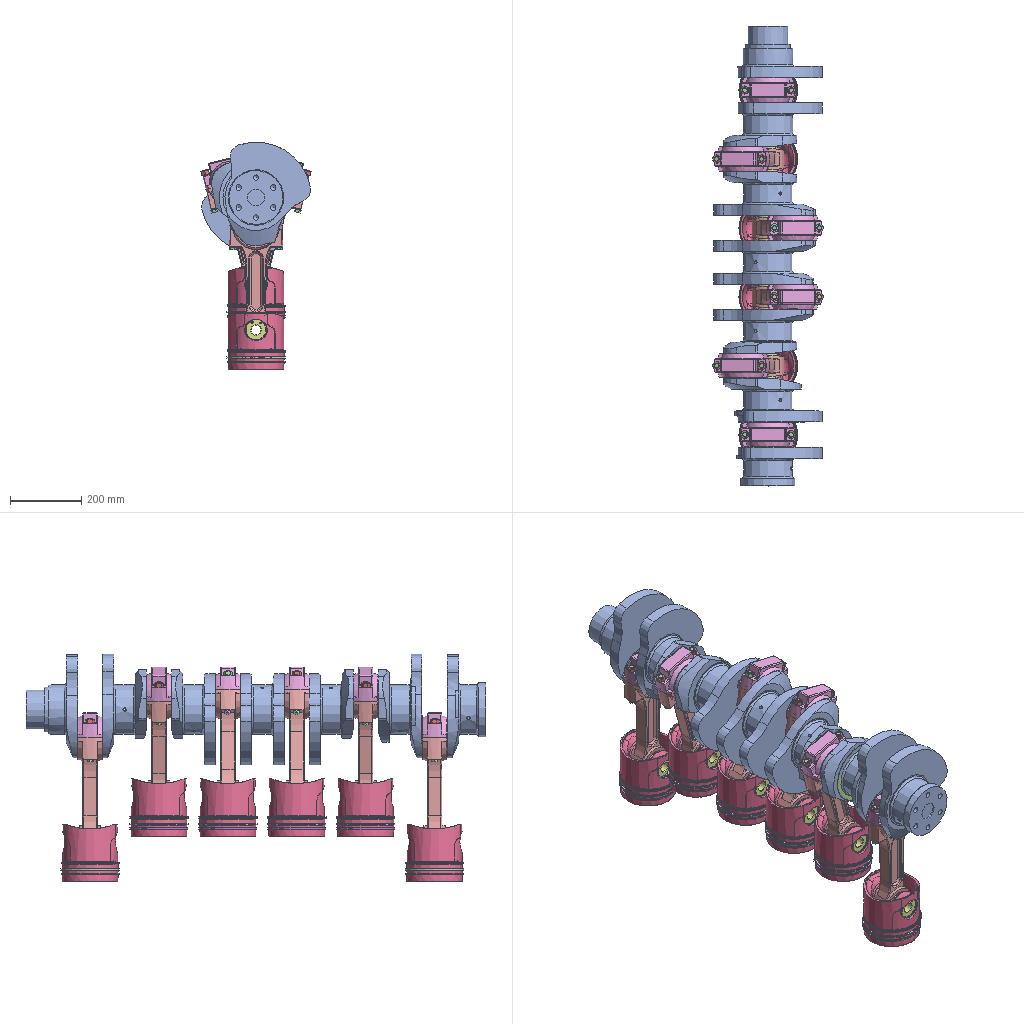Assembly | NX | 16 different items | 109 placed | box 310 x 1294 x 640 mm
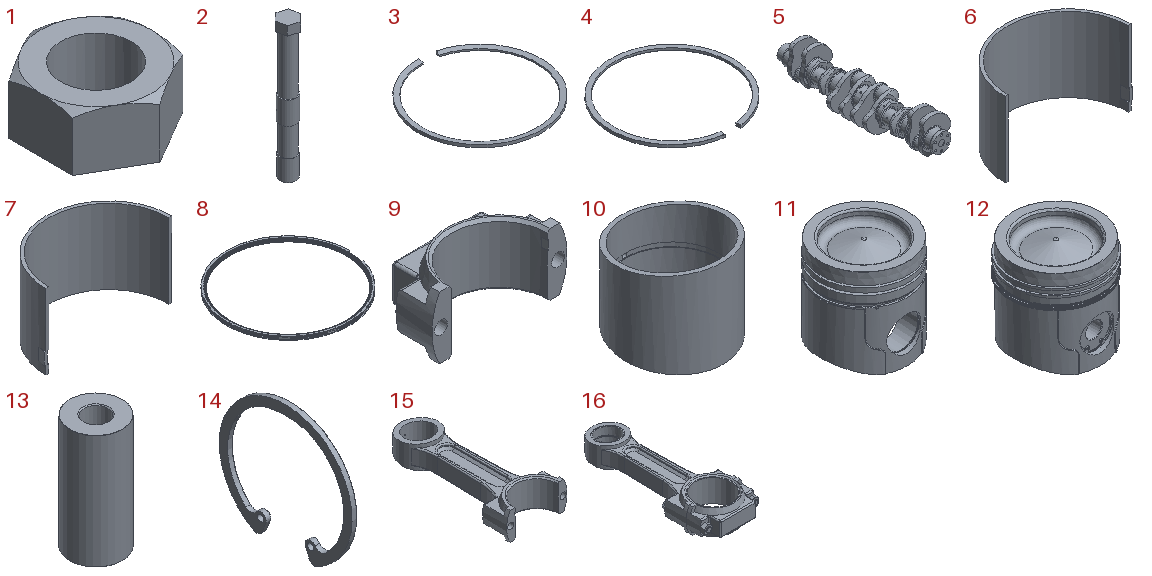Parts list (item | quantity | parent item | size | volume | features):
1 | x12 | in 16 | 22 x 25.403 x 12 mm | 3034 mm3 | features DATUM_CSYS 5, SKETCH 3, EXTRUDE 2, SWP104 1, SYMBOLIC_THREAD 1
2 | x12 | in 16 | 17.119 x 17.607 x 122 mm | 18493 mm3 | features DATUM_CSYS 6, EXTRUDE 4, SKETCH 4, CHAMFER 1, SYMBOLIC_THREAD 1, UNITE 1
3 | x6 | in 12 | 164 x 164 x 3.7 mm | 8808 mm3 | features DATUM_CSYS 2, SKETCH 1, SWP104 1
4 | x6 | in 12 | 164 x 163.314 x 3.7 mm | 10104 mm3 | features DATUM_CSYS 3, EXTRUDE 2, SKETCH 2, BLEND 1, TEXT 1
5 | x1 | - | 306.35 x 1294 x 311.16 mm | 25921208 mm3 | features DATUM_CSYS 74, SKETCH 73, EXTRUDE 53, DATUM_PLANE 19, HOLE PACKAGE 19, SIMPLE HOLE 18, INTERSECTION_CURVES 13, SYMBOLIC_THREAD 12, Instance Feature 10, SKIN 10, SUBTRACT 10, UNITE 9, MIRROR 8, EXTRACT_FACE 6, EXTRACT_STRING 6, MIRROR_SET 3, BLEND 2, CHAMFER 2, Pattern Feature 2, CSUNK_HOLE 1, MOVE_OBJECT 1, SWP104 1
6 | x6 | in 16 | 107.287 x 53 x 63 mm | 25608 mm3 | features DATUM_CSYS 8, SKETCH 6, EXTRUDE 4, DATUM_PLANE 1, UNITE 1
7 | x6 | in 16 | 107.25 x 53 x 63 mm | 25605 mm3 | features DATUM_CSYS 7, SKETCH 5, EXTRUDE 4
8 | x6 | in 12 | 164 x 164 x 4.783 mm | 4407 mm3 | features EXTRACT_STRING 371, Instance Feature 369, SWP104 362, EXTRACT_DATUM_AXIS 360, EXTRUDE 11, DATUM_CSYS 6, SKETCH 5, Pattern Feature 2
9 | x6 | in 16 | 150 x 70 x 69 mm | 212244 mm3 | features DATUM_CSYS 9, SKETCH 7, EXTRUDE 6, BLEND 2, CHAMFER 1, SWP104 1, UNITE 1
10 | x6 | in 16 | 67 x 67 x 57.889 mm | 30363 mm3 | features DATUM_CSYS 5, EXTRUDE 4, SKETCH 4, DATUM_PLANE 2, HOLE PACKAGE 1, MIRROR_SET 1, SIMPLE HOLE 1
11 | x6 | in 12 | 157.8 x 157.8 x 162 mm | 1466782 mm3 | features BLEND 23, EXTRUDE 12, DATUM_CSYS 11, SKETCH 10, HOLE PACKAGE 4, TAPER_HOLE 4, MIRROR_SET 3, SWP104 2, CHAMFER 1, CPROJ 1, DATUM_PLANE 1
12 | x6 | - | 165.688 x 164.309 x 164.424 mm | 1799069 mm3 | features EXTRACT_STRING 371, Instance Feature 369, SWP104 365, EXTRACT_DATUM_AXIS 360, EXTRUDE 27, BLEND 26, DATUM_CSYS 26, SKETCH 20, HOLE PACKAGE 4, TAPER_HOLE 4, MIRROR_SET 3, CHAMFER 2, Pattern Feature 2, CPROJ 1, DATUM_PLANE 1, TEXT 1
13 | x6 | in 12 | 61 x 61 x 132.5 mm | 305546 mm3 | features DATUM_CSYS 2, BLEND 1, CHAMFER 1, EXTRUDE 1, SKETCH 1
14 | x12 | in 12 | 2.4 x 64 x 60.597 mm | 1716 mm3 | features DATUM_CSYS 2, BLEND 1, EXTRUDE 1, SKETCH 1
15 | x6 | in 16 | 150 x 338 x 69 mm | 706906 mm3 | features DATUM_CSYS 13, SKETCH 12, EXTRUDE 10, BLEND 6, CHAMFER 6, UNITE 5, DATUM_PLANE 3, SIMPLE HOLE 3, HOLE PACKAGE 2, MIRROR 2, MIRROR_SET 2, SWP104 2, TRIM BODY 1
16 | x6 | - | 152 x 408 x 69 mm | 1043781 mm3 | features DATUM_CSYS 53, SKETCH 41, EXTRUDE 34, BLEND 8, CHAMFER 8, UNITE 8, DATUM_PLANE 6, SIMPLE HOLE 4, SWP104 4, HOLE PACKAGE 3, MIRROR_SET 3, MIRROR 2, SYMBOLIC_THREAD 2, TRIM BODY 1
Mates (type | each side: item.copy, entity, surface, feature):
In the top assembly
Fix | 5.1 component | 2 times
Touch | 6.1 face cylinder Extrude(2) | 5.1 face cylinder Extrude(48)
Center22 | 15.1 face plane Mirror Body(30) | 15.1 face plane Extrude(4) | 5.1 face plane Extrude(43) | 5.1 face plane Extrude(65)
Touch | 11.1 face cylinder Revolve(2) | assembly line | 3 times
Touch | 13.1 face cylinder Extrude(1) | 10.1 face cylinder Extrude(1) | 5 times
Touch | 7.1 face cylinder Extrude(2) | 5.1 face cylinder Extrude(14)
Center22 | 15.1 face plane Extrude(4) | 15.1 face plane Mirror Body(30) | 5.1 face plane Extrude(18) | 5.1 face plane Extrude(8)
Touch | 11.1 face cylinder Extrude(37) | assembly line
Touch | 7.1 face cylinder Extrude(2) | 5.1 face cylinder Extrude(81)
Center22 | 15.1 face plane Extrude(4) | 15.1 face plane Mirror Body(30) | 5.1 face plane Extrude(77) | 5.1 face plane Mirror Body(90)
Touch | 11.1 face cone Revolve(2) | assembly line | 2 times
Touch | 15.1 face cone Chamfer(36) | 5.1 face cylinder Mirror Body(113)
Center22 | 15.1 face plane Mirror Body(30) | 15.1 face plane Extrude(4) | 5.1 face plane Mirror Body(111) | 5.1 face plane Mirror Body(116)
Touch | 7.1 face cylinder Extrude(2) | 5.1 face cylinder Mirror Body(128)
Touch | 10.1 face cylinder Extrude(1) | 13.1 face cylinder Extrude(1)
Center22 | 15.1 face plane Mirror Body(30) | 15.1 face plane Extrude(4) | 5.1 face plane Extrude(123) | 5.1 face plane Extrude(130)
Touch | 6.1 face cylinder Extrude(2) | 5.1 face cylinder Extrude(101)
Center22 | 15.1 face plane Mirror Body(30) | 15.1 face plane Extrude(4) | 5.1 face plane Mirror Body(109) | 5.1 face plane Extrude(96)
Touch | 15.1 face cylinder Extrude(5) | 13.1 face cylinder Extrude(1)
In subassembly 12
Touch | 14.1 | 11.1 | 3 times
Touch | 13.1 | 11.1 | 2 times
Touch | 14.1 | 13.1
Touch | 3.1 | 11.1 | 2 times
Touch | 4.1 | 11.1 | 2 times
Touch | 8.1 | 11.1
In subassembly 16
Touch | 10.1 | 15.1 | 2 times
Touch | 6.1 | 15.1 | 3 times
Touch | 9.1 | 6.1
Touch | 9.1 | 15.1 | 2 times
Touch | 7.1 | 9.1 | 2 times
Touch | 7.1 | 6.1
Touch | 2.1 | 15.1 | 4 times
Touch | 1.1 | 2.1 | 2 times
Touch | 1.1 | 9.1 | 2 times
Parallel | 1.1 | 9.1 | 2 times